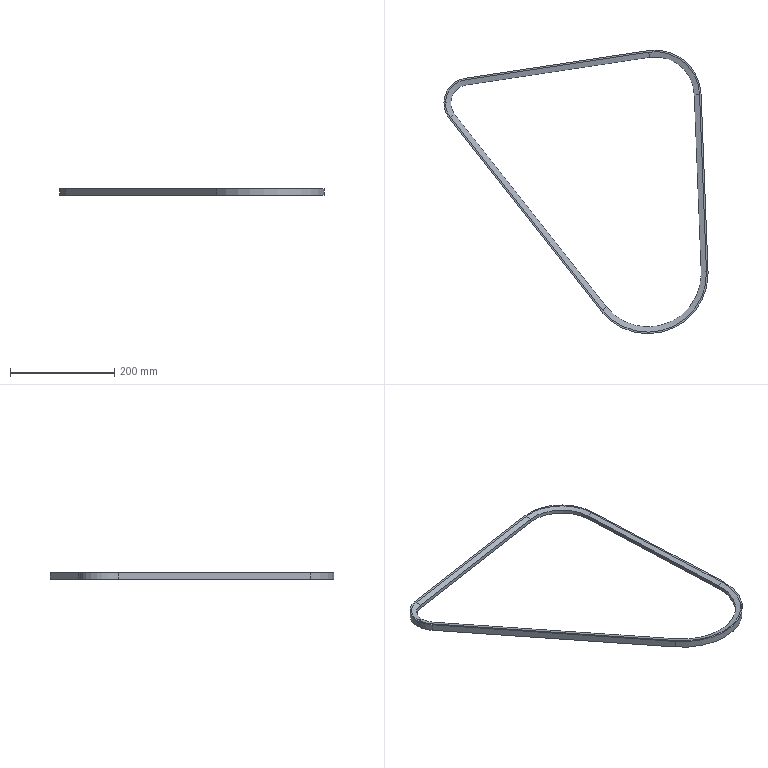Part | SolidWorks | features BaseBody 1 | 1 solid | 30 faces | box 505.859 x 543.35 x 13 mm | volume 231292 mm3 | plane 14 | cylinder 8 | cone 8 | commonest cylinder face diameters 204 x2 230 x2 70 x1 96 x1 149.5 x1 175.5 x1
STEP:
#1=CARTESIAN_POINT('',(4015.899,485.511,10.));
#2=VERTEX_POINT('',#1);
#3=CARTESIAN_POINT('',(4198.023,548.631,10.));
#4=VERTEX_POINT('',#3);
#5=CARTESIAN_POINT('',(4096.023,548.631,10.));
#6=DIRECTION('',(0.,0.,1.));
#7=DIRECTION('',(1.,0.,0.));
#8=AXIS2_PLACEMENT_3D('',#5,#6,#7);
#9=CIRCLE('',#8,102.);
#10=EDGE_CURVE('',#2,#4,#9,.T.);
#11=ORIENTED_EDGE('',*,*,#10,.T.);
#12=CARTESIAN_POINT('',(4198.023,548.631,3.));
#13=VERTEX_POINT('',#12);
#14=CARTESIAN_POINT('',(4198.023,548.631,13.));
#15=DIRECTION('',(0.,0.,-1.));
#16=VECTOR('',#15,1000.);
#17=LINE('',#14,#16);
#18=EDGE_CURVE('',#4,#13,#17,.T.);
#19=ORIENTED_EDGE('',*,*,#18,.T.);
#20=CARTESIAN_POINT('',(4015.899,485.511,3.));
#21=VERTEX_POINT('',#20);
#22=CARTESIAN_POINT('',(4096.023,548.631,3.));
#23=DIRECTION('',(0.,0.,-1.));
#24=DIRECTION('',(1.,0.,0.));
#25=AXIS2_PLACEMENT_3D('',#22,#23,#24);
#26=CIRCLE('',#25,102.);
#27=EDGE_CURVE('',#13,#21,#26,.T.);
#28=ORIENTED_EDGE('',*,*,#27,.T.);
#29=CARTESIAN_POINT('',(4015.899,485.511,13.));
#30=DIRECTION('',(0.,0.,-1.));
#31=VECTOR('',#30,1000.);
#32=LINE('',#29,#31);
#33=EDGE_CURVE('',#2,#21,#32,.T.);
#34=ORIENTED_EDGE('',*,*,#33,.F.);
#35=EDGE_LOOP('',(#11,#19,#28,#34));
#36=FACE_OUTER_BOUND('',#35,.T.);
#37=CARTESIAN_POINT('',(4096.023,548.631,13.));
#38=DIRECTION('',(0.,0.,-1.));
#39=DIRECTION('',(1.,0.,0.));
#40=AXIS2_PLACEMENT_3D('',#37,#38,#39);
#41=CYLINDRICAL_SURFACE('',#40,102.);
#42=ADVANCED_FACE('',(#36),#41,.F.);
#43=CARTESIAN_POINT('',(4211.023,548.631,13.));
#44=VERTEX_POINT('',#43);
#45=CARTESIAN_POINT('',(4210.935,553.109,13.));
#46=VERTEX_POINT('',#45);
#47=CARTESIAN_POINT('',(4096.023,548.631,13.));
#48=DIRECTION('',(0.,0.,1.));
#49=DIRECTION('',(1.,0.,0.));
#50=AXIS2_PLACEMENT_3D('',#47,#48,#49);
#51=CIRCLE('',#50,115.);
#52=EDGE_CURVE('',#44,#46,#51,.T.);
#53=ORIENTED_EDGE('',*,*,#52,.F.);
#54=CARTESIAN_POINT('',(4211.023,548.631,0.));
#55=VERTEX_POINT('',#54);
#56=CARTESIAN_POINT('',(4211.023,548.631,13.));
#57=DIRECTION('',(0.,0.,-1.));
#58=VECTOR('',#57,1000.);
#59=LINE('',#56,#58);
#60=EDGE_CURVE('',#44,#55,#59,.T.);
#61=ORIENTED_EDGE('',*,*,#60,.T.);
#62=CARTESIAN_POINT('',(4210.935,553.109,0.));
#63=VERTEX_POINT('',#62);
#64=CARTESIAN_POINT('',(4096.023,548.631,0.));
#65=DIRECTION('',(0.,0.,1.));
#66=DIRECTION('',(1.,0.,0.));
#67=AXIS2_PLACEMENT_3D('',#64,#65,#66);
#68=CIRCLE('',#67,115.);
#69=EDGE_CURVE('',#55,#63,#68,.T.);
#70=ORIENTED_EDGE('',*,*,#69,.T.);
#71=CARTESIAN_POINT('',(4210.935,553.109,13.));
#72=DIRECTION('',(0.,0.,-1.));
#73=VECTOR('',#72,1000.);
#74=LINE('',#71,#73);
#75=EDGE_CURVE('',#46,#63,#74,.T.);
#76=ORIENTED_EDGE('',*,*,#75,.F.);
#77=EDGE_LOOP('',(#53,#61,#70,#76));
#78=FACE_OUTER_BOUND('',#77,.T.);
#79=CARTESIAN_POINT('',(4096.023,548.631,13.));
#80=DIRECTION('',(0.,0.,-1.));
#81=DIRECTION('',(1.,0.,0.));
#82=AXIS2_PLACEMENT_3D('',#79,#80,#81);
#83=CYLINDRICAL_SURFACE('',#82,115.);
#84=ADVANCED_FACE('',(#78),#83,.T.);
#85=CARTESIAN_POINT('',(3718.164,875.577,10.));
#86=VERTEX_POINT('',#85);
#87=CARTESIAN_POINT('',(3725.67,853.918,10.));
#88=VERTEX_POINT('',#87);
#89=CARTESIAN_POINT('',(3753.164,875.577,10.));
#90=DIRECTION('',(0.,0.,1.));
#91=DIRECTION('',(1.,0.,0.));
#92=AXIS2_PLACEMENT_3D('',#89,#90,#91);
#93=CIRCLE('',#92,35.);
#94=EDGE_CURVE('',#86,#88,#93,.T.);
#95=ORIENTED_EDGE('',*,*,#94,.F.);
#96=CARTESIAN_POINT('',(3708.164,875.577,13.));
#97=VERTEX_POINT('',#96);
#98=CARTESIAN_POINT('',(3718.164,875.577,10.));
#99=DIRECTION('',(-0.9578,0.,0.2873));
#100=VECTOR('',#99,1000.);
#101=LINE('',#98,#100);
#102=EDGE_CURVE('',#86,#97,#101,.T.);
#103=ORIENTED_EDGE('',*,*,#102,.T.);
#104=CARTESIAN_POINT('',(3717.815,847.729,13.));
#105=VERTEX_POINT('',#104);
#106=CARTESIAN_POINT('',(3753.164,875.577,13.));
#107=DIRECTION('',(0.,0.,-1.));
#108=DIRECTION('',(1.,0.,0.));
#109=AXIS2_PLACEMENT_3D('',#106,#107,#108);
#110=CIRCLE('',#109,45.);
#111=EDGE_CURVE('',#105,#97,#110,.T.);
#112=ORIENTED_EDGE('',*,*,#111,.F.);
#113=CARTESIAN_POINT('',(3725.67,853.918,10.));
#114=DIRECTION('',(-0.7524,-0.5927,0.2873));
#115=VECTOR('',#114,1000.);
#116=LINE('',#113,#115);
#117=EDGE_CURVE('',#88,#105,#116,.T.);
#118=ORIENTED_EDGE('',*,*,#117,.F.);
#119=EDGE_LOOP('',(#95,#103,#112,#118));
#120=FACE_OUTER_BOUND('',#119,.T.);
#121=CARTESIAN_POINT('',(3753.164,875.577,10.));
#122=DIRECTION('',(0.,0.,1.));
#123=DIRECTION('',(-1.,0.,0.));
#124=AXIS2_PLACEMENT_3D('',#121,#122,#123);
#125=CONICAL_SURFACE('',#124,35.,1.279);
#126=ADVANCED_FACE('',(#120),#125,.F.);
#127=ORIENTED_EDGE('',*,*,#27,.F.);
#128=CARTESIAN_POINT('',(4208.023,548.631,0.));
#129=VERTEX_POINT('',#128);
#130=CARTESIAN_POINT('',(4208.023,548.631,0.));
#131=DIRECTION('',(0.9578,0.,-0.2873));
#132=VECTOR('',#131,1000.);
#133=LINE('',#130,#132);
#134=EDGE_CURVE('',#13,#129,#133,.T.);
#135=ORIENTED_EDGE('',*,*,#134,.T.);
#136=CARTESIAN_POINT('',(4008.044,479.322,0.));
#137=VERTEX_POINT('',#136);
#138=CARTESIAN_POINT('',(4096.023,548.631,0.));
#139=DIRECTION('',(0.,0.,1.));
#140=DIRECTION('',(1.,0.,0.));
#141=AXIS2_PLACEMENT_3D('',#138,#139,#140);
#142=CIRCLE('',#141,112.);
#143=EDGE_CURVE('',#137,#129,#142,.T.);
#144=ORIENTED_EDGE('',*,*,#143,.F.);
#145=CARTESIAN_POINT('',(4015.899,485.511,3.));
#146=DIRECTION('',(-0.7524,-0.5927,-0.2873));
#147=VECTOR('',#146,1000.);
#148=LINE('',#145,#147);
#149=EDGE_CURVE('',#21,#137,#148,.T.);
#150=ORIENTED_EDGE('',*,*,#149,.F.);
#151=EDGE_LOOP('',(#127,#135,#144,#150));
#152=FACE_OUTER_BOUND('',#151,.T.);
#153=CARTESIAN_POINT('',(4096.023,548.631,0.));
#154=DIRECTION('',(0.,0.,-1.));
#155=DIRECTION('',(1.,0.,0.));
#156=AXIS2_PLACEMENT_3D('',#153,#154,#155);
#157=CONICAL_SURFACE('',#156,112.,1.279);
#158=ADVANCED_FACE('',(#152),#157,.F.);
#159=CARTESIAN_POINT('',(3746.449,920.073,0.));
#160=VERTEX_POINT('',#159);
#161=CARTESIAN_POINT('',(3747.941,910.185,3.));
#162=VERTEX_POINT('',#161);
#163=CARTESIAN_POINT('',(3746.449,920.073,0.));
#164=DIRECTION('',(0.1429,-0.9471,0.2873));
#165=VECTOR('',#164,1000.);
#166=LINE('',#163,#165);
#167=EDGE_CURVE('',#160,#162,#166,.T.);
#168=ORIENTED_EDGE('',*,*,#167,.T.);
#169=CARTESIAN_POINT('',(3725.67,853.918,3.));
#170=VERTEX_POINT('',#169);
#171=CARTESIAN_POINT('',(3753.164,875.577,3.));
#172=DIRECTION('',(0.,0.,-1.));
#173=DIRECTION('',(1.,0.,0.));
#174=AXIS2_PLACEMENT_3D('',#171,#172,#173);
#175=CIRCLE('',#174,35.);
#176=EDGE_CURVE('',#170,#162,#175,.T.);
#177=ORIENTED_EDGE('',*,*,#176,.F.);
#178=CARTESIAN_POINT('',(3717.815,847.729,0.));
#179=VERTEX_POINT('',#178);
#180=CARTESIAN_POINT('',(3725.67,853.918,3.));
#181=DIRECTION('',(-0.7524,-0.5927,-0.2873));
#182=VECTOR('',#181,1000.);
#183=LINE('',#180,#182);
#184=EDGE_CURVE('',#170,#179,#183,.T.);
#185=ORIENTED_EDGE('',*,*,#184,.T.);
#186=CARTESIAN_POINT('',(3753.164,875.577,0.));
#187=DIRECTION('',(0.,0.,1.));
#188=DIRECTION('',(1.,0.,0.));
#189=AXIS2_PLACEMENT_3D('',#186,#187,#188);
#190=CIRCLE('',#189,45.);
#191=EDGE_CURVE('',#160,#179,#190,.T.);
#192=ORIENTED_EDGE('',*,*,#191,.F.);
#193=EDGE_LOOP('',(#168,#177,#185,#192));
#194=FACE_OUTER_BOUND('',#193,.T.);
#195=CARTESIAN_POINT('',(3753.164,875.577,0.));
#196=DIRECTION('',(0.,0.,-1.));
#197=DIRECTION('',(1.,0.,0.));
#198=AXIS2_PLACEMENT_3D('',#195,#196,#197);
#199=CONICAL_SURFACE('',#198,45.,1.279);
#200=ADVANCED_FACE('',(#194),#199,.F.);
#201=ORIENTED_EDGE('',*,*,#149,.T.);
#202=CARTESIAN_POINT('',(4008.044,479.322,0.));
#203=DIRECTION('',(0.6188,-0.7855,0.));
#204=VECTOR('',#203,1000.);
#205=LINE('',#202,#204);
#206=EDGE_CURVE('',#179,#137,#205,.T.);
#207=ORIENTED_EDGE('',*,*,#206,.F.);
#208=ORIENTED_EDGE('',*,*,#184,.F.);
#209=CARTESIAN_POINT('',(3725.67,853.918,3.));
#210=DIRECTION('',(-0.6188,0.7855,0.));
#211=VECTOR('',#210,1000.);
#212=LINE('',#209,#211);
#213=EDGE_CURVE('',#21,#170,#212,.T.);
#214=ORIENTED_EDGE('',*,*,#213,.F.);
#215=EDGE_LOOP('',(#201,#207,#208,#214));
#216=FACE_OUTER_BOUND('',#215,.T.);
#217=CARTESIAN_POINT('',(4008.044,479.322,0.));
#218=DIRECTION('',(0.2257,0.1778,-0.9578));
#219=DIRECTION('',(0.,-0.9832,-0.1825));
#220=AXIS2_PLACEMENT_3D('',#217,#218,#219);
#221=PLANE('',#220);
#222=ADVANCED_FACE('',(#216),#221,.T.);
#223=CARTESIAN_POINT('',(4097.376,973.033,0.));
#224=VERTEX_POINT('',#223);
#225=CARTESIAN_POINT('',(4098.868,963.144,3.));
#226=VERTEX_POINT('',#225);
#227=CARTESIAN_POINT('',(4097.376,973.033,0.));
#228=DIRECTION('',(0.1429,-0.9471,0.2873));
#229=VECTOR('',#228,1000.);
#230=LINE('',#227,#229);
#231=EDGE_CURVE('',#224,#226,#230,.T.);
#232=ORIENTED_EDGE('',*,*,#231,.T.);
#233=CARTESIAN_POINT('',(4098.868,963.144,3.));
#234=DIRECTION('',(0.9888,0.1492,0.));
#235=VECTOR('',#234,1000.);
#236=LINE('',#233,#235);
#237=EDGE_CURVE('',#162,#226,#236,.T.);
#238=ORIENTED_EDGE('',*,*,#237,.F.);
#239=ORIENTED_EDGE('',*,*,#167,.F.);
#240=CARTESIAN_POINT('',(3746.449,920.073,0.));
#241=DIRECTION('',(-0.9888,-0.1492,0.));
#242=VECTOR('',#241,1000.);
#243=LINE('',#240,#242);
#244=EDGE_CURVE('',#224,#160,#243,.T.);
#245=ORIENTED_EDGE('',*,*,#244,.F.);
#246=EDGE_LOOP('',(#232,#238,#239,#245));
#247=FACE_OUTER_BOUND('',#246,.T.);
#248=CARTESIAN_POINT('',(4033.431,963.382,0.));
#249=DIRECTION('',(0.04288,-0.2841,-0.9578));
#250=DIRECTION('',(0.,-0.9587,0.2844));
#251=AXIS2_PLACEMENT_3D('',#248,#249,#250);
#252=PLANE('',#251);
#253=ADVANCED_FACE('',(#247),#252,.T.);
#254=ORIENTED_EDGE('',*,*,#134,.F.);
#255=CARTESIAN_POINT('',(4197.945,552.603,3.));
#256=VERTEX_POINT('',#255);
#257=CARTESIAN_POINT('',(4096.023,548.631,3.));
#258=DIRECTION('',(0.,0.,-1.));
#259=DIRECTION('',(1.,0.,0.));
#260=AXIS2_PLACEMENT_3D('',#257,#258,#259);
#261=CIRCLE('',#260,102.);
#262=EDGE_CURVE('',#256,#13,#261,.T.);
#263=ORIENTED_EDGE('',*,*,#262,.F.);
#264=CARTESIAN_POINT('',(4207.938,552.992,0.));
#265=VERTEX_POINT('',#264);
#266=CARTESIAN_POINT('',(4197.945,552.603,3.));
#267=DIRECTION('',(0.9571,0.03729,-0.2873));
#268=VECTOR('',#267,1000.);
#269=LINE('',#266,#268);
#270=EDGE_CURVE('',#256,#265,#269,.T.);
#271=ORIENTED_EDGE('',*,*,#270,.T.);
#272=CARTESIAN_POINT('',(4096.023,548.631,0.));
#273=DIRECTION('',(0.,0.,1.));
#274=DIRECTION('',(1.,0.,0.));
#275=AXIS2_PLACEMENT_3D('',#272,#273,#274);
#276=CIRCLE('',#275,112.);
#277=EDGE_CURVE('',#129,#265,#276,.T.);
#278=ORIENTED_EDGE('',*,*,#277,.F.);
#279=EDGE_LOOP('',(#254,#263,#271,#278));
#280=FACE_OUTER_BOUND('',#279,.T.);
#281=CARTESIAN_POINT('',(4096.023,548.631,0.));
#282=DIRECTION('',(0.,0.,-1.));
#283=DIRECTION('',(1.,0.,0.));
#284=AXIS2_PLACEMENT_3D('',#281,#282,#283);
#285=CONICAL_SURFACE('',#284,112.,1.279);
#286=ADVANCED_FACE('',(#280),#285,.F.);
#287=CARTESIAN_POINT('',(4194.708,892.531,0.));
#288=VERTEX_POINT('',#287);
#289=CARTESIAN_POINT('',(4184.716,892.142,3.));
#290=VERTEX_POINT('',#289);
#291=CARTESIAN_POINT('',(4194.708,892.531,0.));
#292=DIRECTION('',(-0.9571,-0.03729,0.2873));
#293=VECTOR('',#292,1000.);
#294=LINE('',#291,#293);
#295=EDGE_CURVE('',#288,#290,#294,.T.);
#296=ORIENTED_EDGE('',*,*,#295,.T.);
#297=CARTESIAN_POINT('',(4110.023,889.231,3.));
#298=DIRECTION('',(0.,0.,-1.));
#299=DIRECTION('',(1.,0.,0.));
#300=AXIS2_PLACEMENT_3D('',#297,#298,#299);
#301=CIRCLE('',#300,74.75);
#302=EDGE_CURVE('',#226,#290,#301,.T.);
#303=ORIENTED_EDGE('',*,*,#302,.F.);
#304=ORIENTED_EDGE('',*,*,#231,.F.);
#305=CARTESIAN_POINT('',(4110.023,889.231,0.));
#306=DIRECTION('',(0.,0.,1.));
#307=DIRECTION('',(1.,0.,0.));
#308=AXIS2_PLACEMENT_3D('',#305,#306,#307);
#309=CIRCLE('',#308,84.75);
#310=EDGE_CURVE('',#288,#224,#309,.T.);
#311=ORIENTED_EDGE('',*,*,#310,.F.);
#312=EDGE_LOOP('',(#296,#303,#304,#311));
#313=FACE_OUTER_BOUND('',#312,.T.);
#314=CARTESIAN_POINT('',(4110.023,889.231,0.));
#315=DIRECTION('',(0.,0.,-1.));
#316=DIRECTION('',(1.,0.,0.));
#317=AXIS2_PLACEMENT_3D('',#314,#315,#316);
#318=CONICAL_SURFACE('',#317,84.75,1.279);
#319=ADVANCED_FACE('',(#313),#318,.F.);
#320=ORIENTED_EDGE('',*,*,#270,.F.);
#321=CARTESIAN_POINT('',(4197.945,552.603,3.));
#322=DIRECTION('',(0.03893,-0.9992,0.));
#323=VECTOR('',#322,1000.);
#324=LINE('',#321,#323);
#325=EDGE_CURVE('',#290,#256,#324,.T.);
#326=ORIENTED_EDGE('',*,*,#325,.F.);
#327=ORIENTED_EDGE('',*,*,#295,.F.);
#328=CARTESIAN_POINT('',(4194.708,892.531,0.));
#329=DIRECTION('',(-0.03893,0.9992,0.));
#330=VECTOR('',#329,1000.);
#331=LINE('',#328,#330);
#332=EDGE_CURVE('',#265,#288,#331,.T.);
#333=ORIENTED_EDGE('',*,*,#332,.F.);
#334=EDGE_LOOP('',(#320,#326,#327,#333));
#335=FACE_OUTER_BOUND('',#334,.T.);
#336=CARTESIAN_POINT('',(4207.938,552.992,0.));
#337=DIRECTION('',(-0.2871,-0.01119,-0.9578));
#338=DIRECTION('',(-0.9579,0.,0.2871));
#339=AXIS2_PLACEMENT_3D('',#336,#337,#338);
#340=PLANE('',#339);
#341=ADVANCED_FACE('',(#335),#340,.T.);
#342=CARTESIAN_POINT('',(4197.945,552.603,10.));
#343=VERTEX_POINT('',#342);
#344=CARTESIAN_POINT('',(4207.938,552.992,13.));
#345=VERTEX_POINT('',#344);
#346=CARTESIAN_POINT('',(4197.945,552.603,10.));
#347=DIRECTION('',(0.9571,0.03729,0.2873));
#348=VECTOR('',#347,1000.);
#349=LINE('',#346,#348);
#350=EDGE_CURVE('',#343,#345,#349,.T.);
#351=ORIENTED_EDGE('',*,*,#350,.T.);
#352=CARTESIAN_POINT('',(4194.708,892.531,13.));
#353=VERTEX_POINT('',#352);
#354=CARTESIAN_POINT('',(4207.938,552.992,13.));
#355=DIRECTION('',(0.03893,-0.9992,0.));
#356=VECTOR('',#355,1000.);
#357=LINE('',#354,#356);
#358=EDGE_CURVE('',#353,#345,#357,.T.);
#359=ORIENTED_EDGE('',*,*,#358,.F.);
#360=CARTESIAN_POINT('',(4184.716,892.142,10.));
#361=VERTEX_POINT('',#360);
#362=CARTESIAN_POINT('',(4194.708,892.531,13.));
#363=DIRECTION('',(-0.9571,-0.03729,-0.2873));
#364=VECTOR('',#363,1000.);
#365=LINE('',#362,#364);
#366=EDGE_CURVE('',#353,#361,#365,.T.);
#367=ORIENTED_EDGE('',*,*,#366,.T.);
#368=CARTESIAN_POINT('',(4197.945,552.603,10.));
#369=DIRECTION('',(-0.03893,0.9992,0.));
#370=VECTOR('',#369,1000.);
#371=LINE('',#368,#370);
#372=EDGE_CURVE('',#343,#361,#371,.T.);
#373=ORIENTED_EDGE('',*,*,#372,.F.);
#374=EDGE_LOOP('',(#351,#359,#367,#373));
#375=FACE_OUTER_BOUND('',#374,.T.);
#376=CARTESIAN_POINT('',(4197.945,552.603,10.));
#377=DIRECTION('',(0.2871,0.01119,-0.9578));
#378=DIRECTION('',(0.,-0.9999,-0.01168));
#379=AXIS2_PLACEMENT_3D('',#376,#377,#378);
#380=PLANE('',#379);
#381=ADVANCED_FACE('',(#375),#380,.F.);
#382=CARTESIAN_POINT('',(4097.376,973.033,13.));
#383=VERTEX_POINT('',#382);
#384=CARTESIAN_POINT('',(4098.868,963.144,10.));
#385=VERTEX_POINT('',#384);
#386=CARTESIAN_POINT('',(4097.376,973.033,13.));
#387=DIRECTION('',(0.1429,-0.9471,-0.2873));
#388=VECTOR('',#387,1000.);
#389=LINE('',#386,#388);
#390=EDGE_CURVE('',#383,#385,#389,.T.);
#391=ORIENTED_EDGE('',*,*,#390,.T.);
#392=CARTESIAN_POINT('',(4110.023,889.231,10.));
#393=DIRECTION('',(0.,0.,1.));
#394=DIRECTION('',(1.,0.,0.));
#395=AXIS2_PLACEMENT_3D('',#392,#393,#394);
#396=CIRCLE('',#395,74.75);
#397=EDGE_CURVE('',#361,#385,#396,.T.);
#398=ORIENTED_EDGE('',*,*,#397,.F.);
#399=ORIENTED_EDGE('',*,*,#366,.F.);
#400=CARTESIAN_POINT('',(4110.023,889.231,13.));
#401=DIRECTION('',(0.,0.,-1.));
#402=DIRECTION('',(1.,0.,0.));
#403=AXIS2_PLACEMENT_3D('',#400,#401,#402);
#404=CIRCLE('',#403,84.75);
#405=EDGE_CURVE('',#383,#353,#404,.T.);
#406=ORIENTED_EDGE('',*,*,#405,.F.);
#407=EDGE_LOOP('',(#391,#398,#399,#406));
#408=FACE_OUTER_BOUND('',#407,.T.);
#409=CARTESIAN_POINT('',(4110.023,889.231,10.));
#410=DIRECTION('',(0.,0.,1.));
#411=DIRECTION('',(-1.,0.,0.));
#412=AXIS2_PLACEMENT_3D('',#409,#410,#411);
#413=CONICAL_SURFACE('',#412,74.75,1.279);
#414=ADVANCED_FACE('',(#408),#413,.F.);
#415=CARTESIAN_POINT('',(4008.044,479.322,13.));
#416=VERTEX_POINT('',#415);
#417=CARTESIAN_POINT('',(4015.899,485.511,10.));
#418=DIRECTION('',(-0.7524,-0.5927,0.2873));
#419=VECTOR('',#418,1000.);
#420=LINE('',#417,#419);
#421=EDGE_CURVE('',#2,#416,#420,.T.);
#422=ORIENTED_EDGE('',*,*,#421,.T.);
#423=CARTESIAN_POINT('',(4096.023,548.631,13.));
#424=DIRECTION('',(0.,0.,-1.));
#425=DIRECTION('',(1.,0.,0.));
#426=AXIS2_PLACEMENT_3D('',#423,#424,#425);
#427=CIRCLE('',#426,112.);
#428=EDGE_CURVE('',#345,#416,#427,.T.);
#429=ORIENTED_EDGE('',*,*,#428,.F.);
#430=ORIENTED_EDGE('',*,*,#350,.F.);
#431=CARTESIAN_POINT('',(4096.023,548.631,10.));
#432=DIRECTION('',(0.,0.,1.));
#433=DIRECTION('',(1.,0.,0.));
#434=AXIS2_PLACEMENT_3D('',#431,#432,#433);
#435=CIRCLE('',#434,102.);
#436=EDGE_CURVE('',#4,#343,#435,.T.);
#437=ORIENTED_EDGE('',*,*,#436,.F.);
#438=ORIENTED_EDGE('',*,*,#10,.F.);
#439=EDGE_LOOP('',(#422,#429,#430,#437,#438));
#440=FACE_OUTER_BOUND('',#439,.T.);
#441=CARTESIAN_POINT('',(4096.023,548.631,10.));
#442=DIRECTION('',(0.,0.,1.));
#443=DIRECTION('',(-1.,0.,0.));
#444=AXIS2_PLACEMENT_3D('',#441,#442,#443);
#445=CONICAL_SURFACE('',#444,102.,1.279);
#446=ADVANCED_FACE('',(#440),#445,.F.);
#447=CARTESIAN_POINT('',(3746.449,920.073,13.));
#448=VERTEX_POINT('',#447);
#449=CARTESIAN_POINT('',(3747.941,910.185,10.));
#450=VERTEX_POINT('',#449);
#451=CARTESIAN_POINT('',(3746.449,920.073,13.));
#452=DIRECTION('',(0.1429,-0.9471,-0.2873));
#453=VECTOR('',#452,1000.);
#454=LINE('',#451,#453);
#455=EDGE_CURVE('',#448,#450,#454,.T.);
#456=ORIENTED_EDGE('',*,*,#455,.T.);
#457=CARTESIAN_POINT('',(4098.868,963.144,10.));
#458=DIRECTION('',(-0.9888,-0.1492,0.));
#459=VECTOR('',#458,1000.);
#460=LINE('',#457,#459);
#461=EDGE_CURVE('',#385,#450,#460,.T.);
#462=ORIENTED_EDGE('',*,*,#461,.F.);
#463=ORIENTED_EDGE('',*,*,#390,.F.);
#464=CARTESIAN_POINT('',(4033.431,963.382,13.));
#465=DIRECTION('',(0.9888,0.1492,0.));
#466=VECTOR('',#465,1000.);
#467=LINE('',#464,#466);
#468=EDGE_CURVE('',#448,#383,#467,.T.);
#469=ORIENTED_EDGE('',*,*,#468,.F.);
#470=EDGE_LOOP('',(#456,#462,#463,#469));
#471=FACE_OUTER_BOUND('',#470,.T.);
#472=CARTESIAN_POINT('',(4098.868,963.144,10.));
#473=DIRECTION('',(-0.04288,0.2841,-0.9578));
#474=DIRECTION('',(-0.999,0.,0.04472));
#475=AXIS2_PLACEMENT_3D('',#472,#473,#474);
#476=PLANE('',#475);
#477=ADVANCED_FACE('',(#471),#476,.F.);
#478=ORIENTED_EDGE('',*,*,#117,.T.);
#479=CARTESIAN_POINT('',(4008.044,479.322,13.));
#480=DIRECTION('',(-0.6188,0.7855,0.));
#481=VECTOR('',#480,1000.);
#482=LINE('',#479,#481);
#483=EDGE_CURVE('',#416,#105,#482,.T.);
#484=ORIENTED_EDGE('',*,*,#483,.F.);
#485=ORIENTED_EDGE('',*,*,#421,.F.);
#486=CARTESIAN_POINT('',(3725.67,853.918,10.));
#487=DIRECTION('',(0.6188,-0.7855,0.));
#488=VECTOR('',#487,1000.);
#489=LINE('',#486,#488);
#490=EDGE_CURVE('',#88,#2,#489,.T.);
#491=ORIENTED_EDGE('',*,*,#490,.F.);
#492=EDGE_LOOP('',(#478,#484,#485,#491));
#493=FACE_OUTER_BOUND('',#492,.T.);
#494=CARTESIAN_POINT('',(3725.67,853.918,10.));
#495=DIRECTION('',(-0.2257,-0.1778,-0.9578));
#496=DIRECTION('',(-0.9733,0.,0.2294));
#497=AXIS2_PLACEMENT_3D('',#494,#495,#496);
#498=PLANE('',#497);
#499=ADVANCED_FACE('',(#493),#498,.F.);
#500=ORIENTED_EDGE('',*,*,#102,.F.);
#501=CARTESIAN_POINT('',(3753.164,875.577,10.));
#502=DIRECTION('',(0.,0.,1.));
#503=DIRECTION('',(1.,0.,0.));
#504=AXIS2_PLACEMENT_3D('',#501,#502,#503);
#505=CIRCLE('',#504,35.);
#506=EDGE_CURVE('',#450,#86,#505,.T.);
#507=ORIENTED_EDGE('',*,*,#506,.F.);
#508=ORIENTED_EDGE('',*,*,#455,.F.);
#509=CARTESIAN_POINT('',(3753.164,875.577,13.));
#510=DIRECTION('',(0.,0.,-1.));
#511=DIRECTION('',(1.,0.,0.));
#512=AXIS2_PLACEMENT_3D('',#509,#510,#511);
#513=CIRCLE('',#512,45.);
#514=EDGE_CURVE('',#97,#448,#513,.T.);
#515=ORIENTED_EDGE('',*,*,#514,.F.);
#516=EDGE_LOOP('',(#500,#507,#508,#515));
#517=FACE_OUTER_BOUND('',#516,.T.);
#518=CARTESIAN_POINT('',(3753.164,875.577,10.));
#519=DIRECTION('',(0.,0.,1.));
#520=DIRECTION('',(-1.,0.,0.));
#521=AXIS2_PLACEMENT_3D('',#518,#519,#520);
#522=CONICAL_SURFACE('',#521,35.,1.279);
#523=ADVANCED_FACE('',(#517),#522,.F.);
#524=CARTESIAN_POINT('',(3715.458,845.873,0.));
#525=VERTEX_POINT('',#524);
#526=CARTESIAN_POINT('',(4005.687,477.466,0.));
#527=VERTEX_POINT('',#526);
#528=CARTESIAN_POINT('',(3715.458,845.873,0.));
#529=DIRECTION('',(0.6188,-0.7855,0.));
#530=VECTOR('',#529,1000.);
#531=LINE('',#528,#530);
#532=EDGE_CURVE('',#525,#527,#531,.T.);
#533=ORIENTED_EDGE('',*,*,#532,.F.);
#534=CARTESIAN_POINT('',(3746.001,923.039,0.));
#535=VERTEX_POINT('',#534);
#536=CARTESIAN_POINT('',(3753.164,875.577,0.));
#537=DIRECTION('',(0.,0.,1.));
#538=DIRECTION('',(1.,0.,0.));
#539=AXIS2_PLACEMENT_3D('',#536,#537,#538);
#540=CIRCLE('',#539,48.);
#541=EDGE_CURVE('',#535,#525,#540,.T.);
#542=ORIENTED_EDGE('',*,*,#541,.F.);
#543=CARTESIAN_POINT('',(4096.928,975.999,0.));
#544=VERTEX_POINT('',#543);
#545=CARTESIAN_POINT('',(4096.928,975.999,0.));
#546=DIRECTION('',(-0.9888,-0.1492,0.));
#547=VECTOR('',#546,1000.);
#548=LINE('',#545,#547);
#549=EDGE_CURVE('',#544,#535,#548,.T.);
#550=ORIENTED_EDGE('',*,*,#549,.F.);
#551=CARTESIAN_POINT('',(4197.706,892.648,0.));
#552=VERTEX_POINT('',#551);
#553=CARTESIAN_POINT('',(4110.023,889.231,0.));
#554=DIRECTION('',(0.,0.,1.));
#555=DIRECTION('',(1.,0.,0.));
#556=AXIS2_PLACEMENT_3D('',#553,#554,#555);
#557=CIRCLE('',#556,87.75);
#558=EDGE_CURVE('',#552,#544,#557,.T.);
#559=ORIENTED_EDGE('',*,*,#558,.F.);
#560=CARTESIAN_POINT('',(4210.935,553.109,0.));
#561=DIRECTION('',(-0.03893,0.9992,0.));
#562=VECTOR('',#561,1000.);
#563=LINE('',#560,#562);
#564=EDGE_CURVE('',#63,#552,#563,.T.);
#565=ORIENTED_EDGE('',*,*,#564,.F.);
#566=ORIENTED_EDGE('',*,*,#69,.F.);
#567=CARTESIAN_POINT('',(4096.023,548.631,0.));
#568=DIRECTION('',(0.,0.,1.));
#569=DIRECTION('',(1.,0.,0.));
#570=AXIS2_PLACEMENT_3D('',#567,#568,#569);
#571=CIRCLE('',#570,115.);
#572=EDGE_CURVE('',#527,#55,#571,.T.);
#573=ORIENTED_EDGE('',*,*,#572,.F.);
#574=EDGE_LOOP('',(#533,#542,#550,#559,#565,#566,#573));
#575=FACE_OUTER_BOUND('',#574,.T.);
#576=ORIENTED_EDGE('',*,*,#244,.T.);
#577=ORIENTED_EDGE('',*,*,#191,.T.);
#578=ORIENTED_EDGE('',*,*,#206,.T.);
#579=ORIENTED_EDGE('',*,*,#143,.T.);
#580=ORIENTED_EDGE('',*,*,#277,.T.);
#581=ORIENTED_EDGE('',*,*,#332,.T.);
#582=ORIENTED_EDGE('',*,*,#310,.T.);
#583=EDGE_LOOP('',(#576,#577,#578,#579,#580,#581,#582));
#584=FACE_BOUND('',#583,.T.);
#585=CARTESIAN_POINT('',(4096.023,548.631,0.));
#586=DIRECTION('',(0.,0.,1.));
#587=DIRECTION('',(1.,0.,0.));
#588=AXIS2_PLACEMENT_3D('',#585,#586,#587);
#589=PLANE('',#588);
#590=ADVANCED_FACE('',(#575,#584),#589,.F.);
#591=CARTESIAN_POINT('',(3715.458,845.873,13.));
#592=VERTEX_POINT('',#591);
#593=CARTESIAN_POINT('',(4005.687,477.466,13.));
#594=VERTEX_POINT('',#593);
#595=CARTESIAN_POINT('',(3715.458,845.873,13.));
#596=DIRECTION('',(0.6188,-0.7855,0.));
#597=VECTOR('',#596,1000.);
#598=LINE('',#595,#597);
#599=EDGE_CURVE('',#592,#594,#598,.T.);
#600=ORIENTED_EDGE('',*,*,#599,.T.);
#601=CARTESIAN_POINT('',(4096.023,548.631,13.));
#602=DIRECTION('',(0.,0.,1.));
#603=DIRECTION('',(1.,0.,0.));
#604=AXIS2_PLACEMENT_3D('',#601,#602,#603);
#605=CIRCLE('',#604,115.);
#606=EDGE_CURVE('',#594,#44,#605,.T.);
#607=ORIENTED_EDGE('',*,*,#606,.T.);
#608=ORIENTED_EDGE('',*,*,#52,.T.);
#609=CARTESIAN_POINT('',(4197.706,892.648,13.));
#610=VERTEX_POINT('',#609);
#611=CARTESIAN_POINT('',(4210.935,553.109,13.));
#612=DIRECTION('',(-0.03893,0.9992,0.));
#613=VECTOR('',#612,1000.);
#614=LINE('',#611,#613);
#615=EDGE_CURVE('',#46,#610,#614,.T.);
#616=ORIENTED_EDGE('',*,*,#615,.T.);
#617=CARTESIAN_POINT('',(4096.928,975.999,13.));
#618=VERTEX_POINT('',#617);
#619=CARTESIAN_POINT('',(4110.023,889.231,13.));
#620=DIRECTION('',(0.,0.,1.));
#621=DIRECTION('',(1.,0.,0.));
#622=AXIS2_PLACEMENT_3D('',#619,#620,#621);
#623=CIRCLE('',#622,87.75);
#624=EDGE_CURVE('',#610,#618,#623,.T.);
#625=ORIENTED_EDGE('',*,*,#624,.T.);
#626=CARTESIAN_POINT('',(3746.001,923.039,13.));
#627=VERTEX_POINT('',#626);
#628=CARTESIAN_POINT('',(4096.928,975.999,13.));
#629=DIRECTION('',(-0.9888,-0.1492,0.));
#630=VECTOR('',#629,1000.);
#631=LINE('',#628,#630);
#632=EDGE_CURVE('',#618,#627,#631,.T.);
#633=ORIENTED_EDGE('',*,*,#632,.T.);
#634=CARTESIAN_POINT('',(3753.164,875.577,13.));
#635=DIRECTION('',(0.,0.,1.));
#636=DIRECTION('',(1.,0.,0.));
#637=AXIS2_PLACEMENT_3D('',#634,#635,#636);
#638=CIRCLE('',#637,48.);
#639=EDGE_CURVE('',#627,#592,#638,.T.);
#640=ORIENTED_EDGE('',*,*,#639,.T.);
#641=EDGE_LOOP('',(#600,#607,#608,#616,#625,#633,#640));
#642=FACE_OUTER_BOUND('',#641,.T.);
#643=ORIENTED_EDGE('',*,*,#405,.T.);
#644=ORIENTED_EDGE('',*,*,#358,.T.);
#645=ORIENTED_EDGE('',*,*,#428,.T.);
#646=ORIENTED_EDGE('',*,*,#483,.T.);
#647=ORIENTED_EDGE('',*,*,#111,.T.);
#648=ORIENTED_EDGE('',*,*,#514,.T.);
#649=ORIENTED_EDGE('',*,*,#468,.T.);
#650=EDGE_LOOP('',(#643,#644,#645,#646,#647,#648,#649));
#651=FACE_BOUND('',#650,.T.);
#652=CARTESIAN_POINT('',(4096.023,548.631,13.));
#653=DIRECTION('',(0.,0.,1.));
#654=DIRECTION('',(1.,0.,0.));
#655=AXIS2_PLACEMENT_3D('',#652,#653,#654);
#656=PLANE('',#655);
#657=ADVANCED_FACE('',(#642,#651),#656,.T.);
#658=ORIENTED_EDGE('',*,*,#33,.T.);
#659=ORIENTED_EDGE('',*,*,#213,.T.);
#660=CARTESIAN_POINT('',(3725.67,853.918,13.));
#661=DIRECTION('',(0.,0.,-1.));
#662=VECTOR('',#661,1000.);
#663=LINE('',#660,#662);
#664=EDGE_CURVE('',#88,#170,#663,.T.);
#665=ORIENTED_EDGE('',*,*,#664,.F.);
#666=ORIENTED_EDGE('',*,*,#490,.T.);
#667=EDGE_LOOP('',(#658,#659,#665,#666));
#668=FACE_OUTER_BOUND('',#667,.T.);
#669=CARTESIAN_POINT('',(3725.67,853.918,13.));
#670=DIRECTION('',(0.7855,0.6188,0.));
#671=DIRECTION('',(0.,0.,-1.));
#672=AXIS2_PLACEMENT_3D('',#669,#670,#671);
#673=PLANE('',#672);
#674=ADVANCED_FACE('',(#668),#673,.T.);
#675=ORIENTED_EDGE('',*,*,#541,.T.);
#676=CARTESIAN_POINT('',(3715.458,845.873,13.));
#677=DIRECTION('',(0.,0.,-1.));
#678=VECTOR('',#677,1000.);
#679=LINE('',#676,#678);
#680=EDGE_CURVE('',#592,#525,#679,.T.);
#681=ORIENTED_EDGE('',*,*,#680,.F.);
#682=ORIENTED_EDGE('',*,*,#639,.F.);
#683=CARTESIAN_POINT('',(3746.001,923.039,13.));
#684=DIRECTION('',(0.,0.,-1.));
#685=VECTOR('',#684,1000.);
#686=LINE('',#683,#685);
#687=EDGE_CURVE('',#627,#535,#686,.T.);
#688=ORIENTED_EDGE('',*,*,#687,.T.);
#689=EDGE_LOOP('',(#675,#681,#682,#688));
#690=FACE_OUTER_BOUND('',#689,.T.);
#691=CARTESIAN_POINT('',(3753.164,875.577,13.));
#692=DIRECTION('',(0.,0.,-1.));
#693=DIRECTION('',(1.,0.,0.));
#694=AXIS2_PLACEMENT_3D('',#691,#692,#693);
#695=CYLINDRICAL_SURFACE('',#694,48.);
#696=ADVANCED_FACE('',(#690),#695,.T.);
#697=ORIENTED_EDGE('',*,*,#549,.T.);
#698=ORIENTED_EDGE('',*,*,#687,.F.);
#699=ORIENTED_EDGE('',*,*,#632,.F.);
#700=CARTESIAN_POINT('',(4096.928,975.999,13.));
#701=DIRECTION('',(0.,0.,-1.));
#702=VECTOR('',#701,1000.);
#703=LINE('',#700,#702);
#704=EDGE_CURVE('',#618,#544,#703,.T.);
#705=ORIENTED_EDGE('',*,*,#704,.T.);
#706=EDGE_LOOP('',(#697,#698,#699,#705));
#707=FACE_OUTER_BOUND('',#706,.T.);
#708=CARTESIAN_POINT('',(4096.928,975.999,13.));
#709=DIRECTION('',(0.1492,-0.9888,0.));
#710=DIRECTION('',(0.,0.,-1.));
#711=AXIS2_PLACEMENT_3D('',#708,#709,#710);
#712=PLANE('',#711);
#713=ADVANCED_FACE('',(#707),#712,.F.);
#714=ORIENTED_EDGE('',*,*,#558,.T.);
#715=ORIENTED_EDGE('',*,*,#704,.F.);
#716=ORIENTED_EDGE('',*,*,#624,.F.);
#717=CARTESIAN_POINT('',(4197.706,892.648,13.));
#718=DIRECTION('',(0.,0.,-1.));
#719=VECTOR('',#718,1000.);
#720=LINE('',#717,#719);
#721=EDGE_CURVE('',#610,#552,#720,.T.);
#722=ORIENTED_EDGE('',*,*,#721,.T.);
#723=EDGE_LOOP('',(#714,#715,#716,#722));
#724=FACE_OUTER_BOUND('',#723,.T.);
#725=CARTESIAN_POINT('',(4110.023,889.231,13.));
#726=DIRECTION('',(0.,0.,-1.));
#727=DIRECTION('',(1.,0.,0.));
#728=AXIS2_PLACEMENT_3D('',#725,#726,#727);
#729=CYLINDRICAL_SURFACE('',#728,87.75);
#730=ADVANCED_FACE('',(#724),#729,.T.);
#731=ORIENTED_EDGE('',*,*,#564,.T.);
#732=ORIENTED_EDGE('',*,*,#721,.F.);
#733=ORIENTED_EDGE('',*,*,#615,.F.);
#734=ORIENTED_EDGE('',*,*,#75,.T.);
#735=EDGE_LOOP('',(#731,#732,#733,#734));
#736=FACE_OUTER_BOUND('',#735,.T.);
#737=CARTESIAN_POINT('',(4210.935,553.109,13.));
#738=DIRECTION('',(-0.9992,-0.03893,0.));
#739=DIRECTION('',(-0.03893,0.9992,0.));
#740=AXIS2_PLACEMENT_3D('',#737,#738,#739);
#741=PLANE('',#740);
#742=ADVANCED_FACE('',(#736),#741,.F.);
#743=ORIENTED_EDGE('',*,*,#60,.F.);
#744=ORIENTED_EDGE('',*,*,#606,.F.);
#745=CARTESIAN_POINT('',(4005.687,477.466,13.));
#746=DIRECTION('',(0.,0.,-1.));
#747=VECTOR('',#746,1000.);
#748=LINE('',#745,#747);
#749=EDGE_CURVE('',#594,#527,#748,.T.);
#750=ORIENTED_EDGE('',*,*,#749,.T.);
#751=ORIENTED_EDGE('',*,*,#572,.T.);
#752=EDGE_LOOP('',(#743,#744,#750,#751));
#753=FACE_OUTER_BOUND('',#752,.T.);
#754=CARTESIAN_POINT('',(4096.023,548.631,13.));
#755=DIRECTION('',(0.,0.,-1.));
#756=DIRECTION('',(1.,0.,0.));
#757=AXIS2_PLACEMENT_3D('',#754,#755,#756);
#758=CYLINDRICAL_SURFACE('',#757,115.);
#759=ADVANCED_FACE('',(#753),#758,.T.);
#760=ORIENTED_EDGE('',*,*,#532,.T.);
#761=ORIENTED_EDGE('',*,*,#749,.F.);
#762=ORIENTED_EDGE('',*,*,#599,.F.);
#763=ORIENTED_EDGE('',*,*,#680,.T.);
#764=EDGE_LOOP('',(#760,#761,#762,#763));
#765=FACE_OUTER_BOUND('',#764,.T.);
#766=CARTESIAN_POINT('',(3715.458,845.873,13.));
#767=DIRECTION('',(0.7855,0.6188,0.));
#768=DIRECTION('',(0.,0.,-1.));
#769=AXIS2_PLACEMENT_3D('',#766,#767,#768);
#770=PLANE('',#769);
#771=ADVANCED_FACE('',(#765),#770,.F.);
#772=ORIENTED_EDGE('',*,*,#18,.F.);
#773=ORIENTED_EDGE('',*,*,#436,.T.);
#774=CARTESIAN_POINT('',(4197.945,552.603,13.));
#775=DIRECTION('',(0.,0.,-1.));
#776=VECTOR('',#775,1000.);
#777=LINE('',#774,#776);
#778=EDGE_CURVE('',#343,#256,#777,.T.);
#779=ORIENTED_EDGE('',*,*,#778,.T.);
#780=ORIENTED_EDGE('',*,*,#262,.T.);
#781=EDGE_LOOP('',(#772,#773,#779,#780));
#782=FACE_OUTER_BOUND('',#781,.T.);
#783=CARTESIAN_POINT('',(4096.023,548.631,13.));
#784=DIRECTION('',(0.,0.,-1.));
#785=DIRECTION('',(1.,0.,0.));
#786=AXIS2_PLACEMENT_3D('',#783,#784,#785);
#787=CYLINDRICAL_SURFACE('',#786,102.);
#788=ADVANCED_FACE('',(#782),#787,.F.);
#789=CARTESIAN_POINT('',(4184.716,892.142,13.));
#790=DIRECTION('',(0.,0.,-1.));
#791=VECTOR('',#790,1000.);
#792=LINE('',#789,#791);
#793=EDGE_CURVE('',#361,#290,#792,.T.);
#794=ORIENTED_EDGE('',*,*,#793,.T.);
#795=ORIENTED_EDGE('',*,*,#325,.T.);
#796=ORIENTED_EDGE('',*,*,#778,.F.);
#797=ORIENTED_EDGE('',*,*,#372,.T.);
#798=EDGE_LOOP('',(#794,#795,#796,#797));
#799=FACE_OUTER_BOUND('',#798,.T.);
#800=CARTESIAN_POINT('',(4197.945,552.603,13.));
#801=DIRECTION('',(-0.9992,-0.03893,0.));
#802=DIRECTION('',(-0.03893,0.9992,0.));
#803=AXIS2_PLACEMENT_3D('',#800,#801,#802);
#804=PLANE('',#803);
#805=ADVANCED_FACE('',(#799),#804,.T.);
#806=CARTESIAN_POINT('',(4098.868,963.144,13.));
#807=DIRECTION('',(0.,0.,-1.));
#808=VECTOR('',#807,1000.);
#809=LINE('',#806,#808);
#810=EDGE_CURVE('',#385,#226,#809,.T.);
#811=ORIENTED_EDGE('',*,*,#810,.T.);
#812=ORIENTED_EDGE('',*,*,#302,.T.);
#813=ORIENTED_EDGE('',*,*,#793,.F.);
#814=ORIENTED_EDGE('',*,*,#397,.T.);
#815=EDGE_LOOP('',(#811,#812,#813,#814));
#816=FACE_OUTER_BOUND('',#815,.T.);
#817=CARTESIAN_POINT('',(4110.023,889.231,13.));
#818=DIRECTION('',(0.,0.,-1.));
#819=DIRECTION('',(1.,0.,0.));
#820=AXIS2_PLACEMENT_3D('',#817,#818,#819);
#821=CYLINDRICAL_SURFACE('',#820,74.75);
#822=ADVANCED_FACE('',(#816),#821,.F.);
#823=CARTESIAN_POINT('',(3747.941,910.185,13.));
#824=DIRECTION('',(0.,0.,-1.));
#825=VECTOR('',#824,1000.);
#826=LINE('',#823,#825);
#827=EDGE_CURVE('',#450,#162,#826,.T.);
#828=ORIENTED_EDGE('',*,*,#827,.T.);
#829=ORIENTED_EDGE('',*,*,#237,.T.);
#830=ORIENTED_EDGE('',*,*,#810,.F.);
#831=ORIENTED_EDGE('',*,*,#461,.T.);
#832=EDGE_LOOP('',(#828,#829,#830,#831));
#833=FACE_OUTER_BOUND('',#832,.T.);
#834=CARTESIAN_POINT('',(4098.868,963.144,13.));
#835=DIRECTION('',(0.1492,-0.9888,0.));
#836=DIRECTION('',(0.,0.,-1.));
#837=AXIS2_PLACEMENT_3D('',#834,#835,#836);
#838=PLANE('',#837);
#839=ADVANCED_FACE('',(#833),#838,.T.);
#840=ORIENTED_EDGE('',*,*,#664,.T.);
#841=ORIENTED_EDGE('',*,*,#176,.T.);
#842=ORIENTED_EDGE('',*,*,#827,.F.);
#843=ORIENTED_EDGE('',*,*,#506,.T.);
#844=ORIENTED_EDGE('',*,*,#94,.T.);
#845=EDGE_LOOP('',(#840,#841,#842,#843,#844));
#846=FACE_OUTER_BOUND('',#845,.T.);
#847=CARTESIAN_POINT('',(3753.164,875.577,13.));
#848=DIRECTION('',(0.,0.,-1.));
#849=DIRECTION('',(1.,0.,0.));
#850=AXIS2_PLACEMENT_3D('',#847,#848,#849);
#851=CYLINDRICAL_SURFACE('',#850,35.);
#852=ADVANCED_FACE('',(#846),#851,.F.);
#853=CLOSED_SHELL('',(#42,#84,#126,#158,#200,#222,#253,#286,#319,#341,#381,#414,#446,#477,#499,#523,#590,#657,#674,#696,#713,#730,#742,#759,#771,#788,#805,#822,#839,#852));
#854=MANIFOLD_SOLID_BREP('',#853);
#855=CARTESIAN_POINT('',(0.,0.,0.));
#856=DIRECTION('',(0.,0.,1.));
#857=DIRECTION('',(1.,0.,0.));
#858=AXIS2_PLACEMENT_3D('',#855,#856,#857);
#859=(LENGTH_UNIT()NAMED_UNIT(*)SI_UNIT(.MILLI.,.METRE.));
#860=UNCERTAINTY_MEASURE_WITH_UNIT(LENGTH_MEASURE(0.00001),#859,'','');
#861=(NAMED_UNIT(*)PLANE_ANGLE_UNIT()SI_UNIT($,.RADIAN.));
#862=(NAMED_UNIT(*)SI_UNIT($,.STERADIAN.)SOLID_ANGLE_UNIT());
#863=(GEOMETRIC_REPRESENTATION_CONTEXT(3)GLOBAL_UNCERTAINTY_ASSIGNED_CONTEXT((#860))GLOBAL_UNIT_ASSIGNED_CONTEXT((#859,#861,#862))REPRESENTATION_CONTEXT('',''));
#864=ADVANCED_BREP_SHAPE_REPRESENTATION('',(#854,#858),#863);